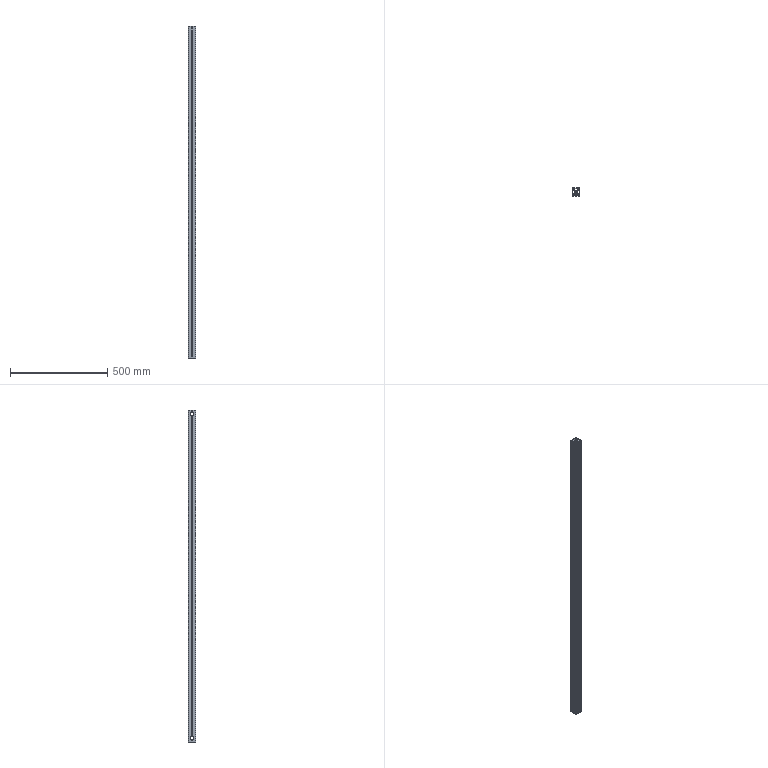Part | SolidWorks | features BaseBody 1, HoleWzd 1, MoveFace 1 | 1 solid | 242 faces | box 40 x 40 x 1705 mm | volume 1001101 mm3 | plane 187 | cylinder 55 | commonest cylinder face diameters 6.8 x15 2 x14 19 x12 1 x6 5 x4 9 x4